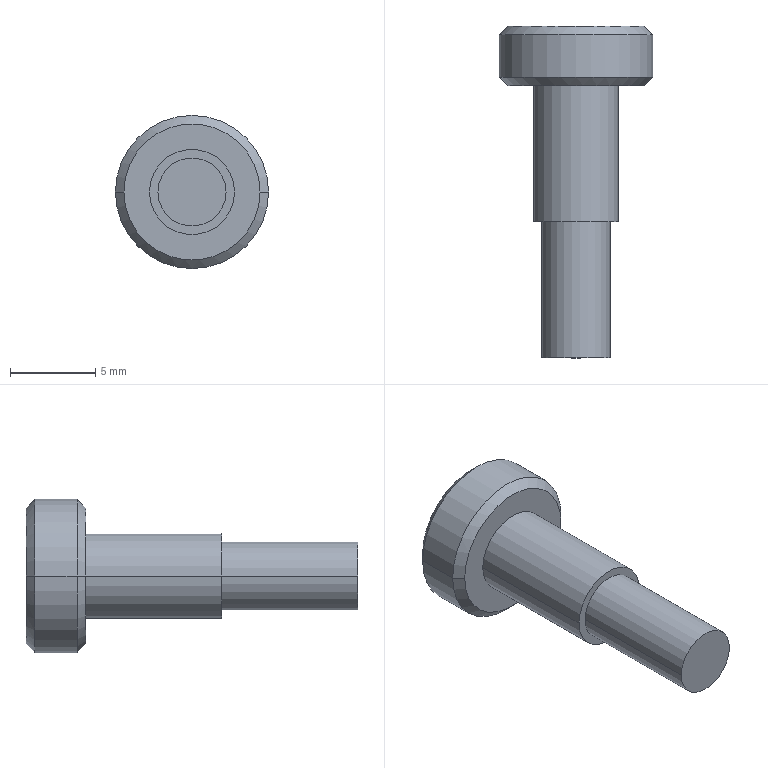Part | SolidWorks | features Attribute 3, Chamfer 1, ICE 1, Revolution 1 | 1 solid | 21 faces | box 9 x 19.5 x 9 mm | volume 457.876 mm3 | plane 11 | cylinder 6 | cone 4 | commonest cylinder face diameters 4 x2 5 x2 9 x2
STEP:
#1=CARTESIAN_POINT('',(-4.,19.5,0.));
#2=VERTEX_POINT('',#1);
#3=CARTESIAN_POINT('',(4.,19.5,0.));
#4=VERTEX_POINT('',#3);
#5=CARTESIAN_POINT('',(0.,19.5,0.));
#6=DIRECTION('',(0.,1.,0.));
#7=DIRECTION('',(1.,0.,0.));
#8=AXIS2_PLACEMENT_3D('',#5,#6,#7);
#9=CIRCLE('',#8,4.);
#10=EDGE_CURVE('',#2,#4,#9,.T.);
#11=ORIENTED_EDGE('',*,*,#10,.F.);
#12=CARTESIAN_POINT('',(-4.5,19.,0.));
#13=VERTEX_POINT('',#12);
#14=CARTESIAN_POINT('',(-4.5,19.,0.));
#15=DIRECTION('',(-0.7071,-0.7071,0.));
#16=VECTOR('',#15,1000.);
#17=LINE('',#14,#16);
#18=EDGE_CURVE('',#2,#13,#17,.T.);
#19=ORIENTED_EDGE('',*,*,#18,.T.);
#20=CARTESIAN_POINT('',(4.5,19.,0.));
#21=VERTEX_POINT('',#20);
#22=CARTESIAN_POINT('',(0.,19.,0.));
#23=DIRECTION('',(0.,-1.,0.));
#24=DIRECTION('',(1.,0.,0.));
#25=AXIS2_PLACEMENT_3D('',#22,#23,#24);
#26=CIRCLE('',#25,4.5);
#27=EDGE_CURVE('',#21,#13,#26,.T.);
#28=ORIENTED_EDGE('',*,*,#27,.F.);
#29=CARTESIAN_POINT('',(4.5,19.,0.));
#30=DIRECTION('',(0.7071,-0.7071,0.));
#31=VECTOR('',#30,1000.);
#32=LINE('',#29,#31);
#33=EDGE_CURVE('',#4,#21,#32,.T.);
#34=ORIENTED_EDGE('',*,*,#33,.F.);
#35=EDGE_LOOP('',(#11,#19,#28,#34));
#36=FACE_OUTER_BOUND('',#35,.T.);
#37=CARTESIAN_POINT('',(0.,19.,0.));
#38=DIRECTION('',(0.,-1.,0.));
#39=DIRECTION('',(1.,0.,0.));
#40=AXIS2_PLACEMENT_3D('',#37,#38,#39);
#41=CONICAL_SURFACE('',#40,4.5,0.7854);
#42=ADVANCED_FACE('',(#36),#41,.T.);
#43=CARTESIAN_POINT('',(4.,16.,0.));
#44=VERTEX_POINT('',#43);
#45=CARTESIAN_POINT('',(-4.,16.,0.));
#46=VERTEX_POINT('',#45);
#47=CARTESIAN_POINT('',(0.,16.,0.));
#48=DIRECTION('',(0.,-1.,0.));
#49=DIRECTION('',(-1.,0.,0.));
#50=AXIS2_PLACEMENT_3D('',#47,#48,#49);
#51=CIRCLE('',#50,4.);
#52=EDGE_CURVE('',#44,#46,#51,.T.);
#53=ORIENTED_EDGE('',*,*,#52,.F.);
#54=CARTESIAN_POINT('',(4.5,16.5,0.));
#55=VERTEX_POINT('',#54);
#56=CARTESIAN_POINT('',(4.,16.,0.));
#57=DIRECTION('',(0.7071,0.7071,0.));
#58=VECTOR('',#57,1000.);
#59=LINE('',#56,#58);
#60=EDGE_CURVE('',#44,#55,#59,.T.);
#61=ORIENTED_EDGE('',*,*,#60,.T.);
#62=CARTESIAN_POINT('',(-4.5,16.5,0.));
#63=VERTEX_POINT('',#62);
#64=CARTESIAN_POINT('',(0.,16.5,0.));
#65=DIRECTION('',(0.,1.,0.));
#66=DIRECTION('',(-1.,0.,0.));
#67=AXIS2_PLACEMENT_3D('',#64,#65,#66);
#68=CIRCLE('',#67,4.5);
#69=EDGE_CURVE('',#63,#55,#68,.T.);
#70=ORIENTED_EDGE('',*,*,#69,.F.);
#71=CARTESIAN_POINT('',(-4.,16.,0.));
#72=DIRECTION('',(-0.7071,0.7071,0.));
#73=VECTOR('',#72,1000.);
#74=LINE('',#71,#73);
#75=EDGE_CURVE('',#46,#63,#74,.T.);
#76=ORIENTED_EDGE('',*,*,#75,.F.);
#77=EDGE_LOOP('',(#53,#61,#70,#76));
#78=FACE_OUTER_BOUND('',#77,.T.);
#79=CARTESIAN_POINT('',(0.,16.,0.));
#80=DIRECTION('',(0.,1.,0.));
#81=DIRECTION('',(-1.,0.,0.));
#82=AXIS2_PLACEMENT_3D('',#79,#80,#81);
#83=CONICAL_SURFACE('',#82,4.,0.7854);
#84=ADVANCED_FACE('',(#78),#83,.T.);
#85=CARTESIAN_POINT('',(2.,8.,0.));
#86=VERTEX_POINT('',#85);
#87=CARTESIAN_POINT('',(-2.,8.,0.));
#88=VERTEX_POINT('',#87);
#89=CARTESIAN_POINT('',(0.,8.,0.));
#90=DIRECTION('',(0.,-1.,0.));
#91=DIRECTION('',(1.,0.,0.));
#92=AXIS2_PLACEMENT_3D('',#89,#90,#91);
#93=CIRCLE('',#92,2.);
#94=EDGE_CURVE('',#86,#88,#93,.T.);
#95=ORIENTED_EDGE('',*,*,#94,.T.);
#96=CARTESIAN_POINT('',(-2.,0.,0.));
#97=VERTEX_POINT('',#96);
#98=CARTESIAN_POINT('',(-2.,0.,0.));
#99=DIRECTION('',(0.,-1.,0.));
#100=VECTOR('',#99,1000.);
#101=LINE('',#98,#100);
#102=EDGE_CURVE('',#88,#97,#101,.T.);
#103=ORIENTED_EDGE('',*,*,#102,.T.);
#104=CARTESIAN_POINT('',(2.,0.,0.));
#105=VERTEX_POINT('',#104);
#106=CARTESIAN_POINT('',(0.,0.,0.));
#107=DIRECTION('',(0.,-1.,0.));
#108=DIRECTION('',(1.,0.,0.));
#109=AXIS2_PLACEMENT_3D('',#106,#107,#108);
#110=CIRCLE('',#109,2.);
#111=EDGE_CURVE('',#105,#97,#110,.T.);
#112=ORIENTED_EDGE('',*,*,#111,.F.);
#113=CARTESIAN_POINT('',(2.,0.,0.));
#114=DIRECTION('',(0.,-1.,0.));
#115=VECTOR('',#114,1000.);
#116=LINE('',#113,#115);
#117=EDGE_CURVE('',#86,#105,#116,.T.);
#118=ORIENTED_EDGE('',*,*,#117,.F.);
#119=EDGE_LOOP('',(#95,#103,#112,#118));
#120=FACE_OUTER_BOUND('',#119,.T.);
#121=CARTESIAN_POINT('',(0.,0.,0.));
#122=DIRECTION('',(0.,-1.,0.));
#123=DIRECTION('',(1.,0.,0.));
#124=AXIS2_PLACEMENT_3D('',#121,#122,#123);
#125=CYLINDRICAL_SURFACE('',#124,2.);
#126=ADVANCED_FACE('',(#120),#125,.T.);
#127=CARTESIAN_POINT('',(2.5,16.,0.));
#128=VERTEX_POINT('',#127);
#129=CARTESIAN_POINT('',(-2.5,16.,0.));
#130=VERTEX_POINT('',#129);
#131=CARTESIAN_POINT('',(0.,16.,0.));
#132=DIRECTION('',(0.,-1.,0.));
#133=DIRECTION('',(1.,0.,0.));
#134=AXIS2_PLACEMENT_3D('',#131,#132,#133);
#135=CIRCLE('',#134,2.5);
#136=EDGE_CURVE('',#128,#130,#135,.T.);
#137=ORIENTED_EDGE('',*,*,#136,.T.);
#138=CARTESIAN_POINT('',(-2.5,8.,0.));
#139=VERTEX_POINT('',#138);
#140=CARTESIAN_POINT('',(-2.5,0.,0.));
#141=DIRECTION('',(0.,-1.,0.));
#142=VECTOR('',#141,1000.);
#143=LINE('',#140,#142);
#144=EDGE_CURVE('',#130,#139,#143,.T.);
#145=ORIENTED_EDGE('',*,*,#144,.T.);
#146=CARTESIAN_POINT('',(2.5,8.,0.));
#147=VERTEX_POINT('',#146);
#148=CARTESIAN_POINT('',(0.,8.,0.));
#149=DIRECTION('',(0.,-1.,0.));
#150=DIRECTION('',(1.,0.,0.));
#151=AXIS2_PLACEMENT_3D('',#148,#149,#150);
#152=CIRCLE('',#151,2.5);
#153=EDGE_CURVE('',#147,#139,#152,.T.);
#154=ORIENTED_EDGE('',*,*,#153,.F.);
#155=CARTESIAN_POINT('',(2.5,0.,0.));
#156=DIRECTION('',(0.,-1.,0.));
#157=VECTOR('',#156,1000.);
#158=LINE('',#155,#157);
#159=EDGE_CURVE('',#128,#147,#158,.T.);
#160=ORIENTED_EDGE('',*,*,#159,.F.);
#161=EDGE_LOOP('',(#137,#145,#154,#160));
#162=FACE_OUTER_BOUND('',#161,.T.);
#163=CARTESIAN_POINT('',(0.,0.,0.));
#164=DIRECTION('',(0.,-1.,0.));
#165=DIRECTION('',(1.,0.,0.));
#166=AXIS2_PLACEMENT_3D('',#163,#164,#165);
#167=CYLINDRICAL_SURFACE('',#166,2.5);
#168=ADVANCED_FACE('',(#162),#167,.T.);
#169=ORIENTED_EDGE('',*,*,#27,.T.);
#170=CARTESIAN_POINT('',(-4.5,0.,0.));
#171=DIRECTION('',(0.,-1.,0.));
#172=VECTOR('',#171,1000.);
#173=LINE('',#170,#172);
#174=EDGE_CURVE('',#13,#63,#173,.T.);
#175=ORIENTED_EDGE('',*,*,#174,.T.);
#176=ORIENTED_EDGE('',*,*,#69,.T.);
#177=CARTESIAN_POINT('',(4.5,0.,0.));
#178=DIRECTION('',(0.,-1.,0.));
#179=VECTOR('',#178,1000.);
#180=LINE('',#177,#179);
#181=EDGE_CURVE('',#21,#55,#180,.T.);
#182=ORIENTED_EDGE('',*,*,#181,.F.);
#183=EDGE_LOOP('',(#169,#175,#176,#182));
#184=FACE_OUTER_BOUND('',#183,.T.);
#185=CARTESIAN_POINT('',(0.,0.,0.));
#186=DIRECTION('',(0.,-1.,0.));
#187=DIRECTION('',(1.,0.,0.));
#188=AXIS2_PLACEMENT_3D('',#185,#186,#187);
#189=CYLINDRICAL_SURFACE('',#188,4.5);
#190=ADVANCED_FACE('',(#184),#189,.T.);
#191=ORIENTED_EDGE('',*,*,#111,.T.);
#192=CARTESIAN_POINT('',(0.,0.,0.));
#193=DIRECTION('',(0.,-1.,0.));
#194=DIRECTION('',(1.,0.,0.));
#195=AXIS2_PLACEMENT_3D('',#192,#193,#194);
#196=CIRCLE('',#195,2.);
#197=EDGE_CURVE('',#97,#105,#196,.T.);
#198=ORIENTED_EDGE('',*,*,#197,.T.);
#199=EDGE_LOOP('',(#191,#198));
#200=FACE_OUTER_BOUND('',#199,.T.);
#201=CARTESIAN_POINT('',(-2.,0.,0.));
#202=DIRECTION('',(0.,1.,0.));
#203=DIRECTION('',(-1.,0.,0.));
#204=AXIS2_PLACEMENT_3D('',#201,#202,#203);
#205=PLANE('',#204);
#206=ADVANCED_FACE('',(#200),#205,.F.);
#207=CARTESIAN_POINT('',(0.,19.5,0.));
#208=DIRECTION('',(0.,1.,0.));
#209=DIRECTION('',(1.,0.,0.));
#210=AXIS2_PLACEMENT_3D('',#207,#208,#209);
#211=CIRCLE('',#210,4.);
#212=EDGE_CURVE('',#4,#2,#211,.T.);
#213=ORIENTED_EDGE('',*,*,#212,.T.);
#214=ORIENTED_EDGE('',*,*,#10,.T.);
#215=EDGE_LOOP('',(#213,#214));
#216=FACE_OUTER_BOUND('',#215,.T.);
#217=CARTESIAN_POINT('',(1.51,19.5,-0.8492));
#218=VERTEX_POINT('',#217);
#219=CARTESIAN_POINT('',(0.01932,19.5,-1.732));
#220=VERTEX_POINT('',#219);
#221=CARTESIAN_POINT('',(1.51,19.5,-0.8492));
#222=DIRECTION('',(-0.8604,0.,-0.5096));
#223=VECTOR('',#222,1000.);
#224=LINE('',#221,#223);
#225=EDGE_CURVE('',#218,#220,#224,.T.);
#226=ORIENTED_EDGE('',*,*,#225,.F.);
#227=CARTESIAN_POINT('',(1.49,19.5,0.8827));
#228=VERTEX_POINT('',#227);
#229=CARTESIAN_POINT('',(1.49,19.5,0.8827));
#230=DIRECTION('',(0.01115,0.,-0.9999));
#231=VECTOR('',#230,1000.);
#232=LINE('',#229,#231);
#233=EDGE_CURVE('',#228,#218,#232,.T.);
#234=ORIENTED_EDGE('',*,*,#233,.F.);
#235=CARTESIAN_POINT('',(-0.01932,19.5,1.732));
#236=VERTEX_POINT('',#235);
#237=CARTESIAN_POINT('',(-0.01932,19.5,1.732));
#238=DIRECTION('',(0.8715,0.,-0.4903));
#239=VECTOR('',#238,1000.);
#240=LINE('',#237,#239);
#241=EDGE_CURVE('',#236,#228,#240,.T.);
#242=ORIENTED_EDGE('',*,*,#241,.F.);
#243=CARTESIAN_POINT('',(-1.51,19.5,0.8492));
#244=VERTEX_POINT('',#243);
#245=CARTESIAN_POINT('',(-1.51,19.5,0.8492));
#246=DIRECTION('',(0.8604,0.,0.5096));
#247=VECTOR('',#246,1000.);
#248=LINE('',#245,#247);
#249=EDGE_CURVE('',#244,#236,#248,.T.);
#250=ORIENTED_EDGE('',*,*,#249,.F.);
#251=CARTESIAN_POINT('',(-1.49,19.5,-0.8827));
#252=VERTEX_POINT('',#251);
#253=CARTESIAN_POINT('',(-1.49,19.5,-0.8827));
#254=DIRECTION('',(-0.01115,0.,0.9999));
#255=VECTOR('',#254,1000.);
#256=LINE('',#253,#255);
#257=EDGE_CURVE('',#252,#244,#256,.T.);
#258=ORIENTED_EDGE('',*,*,#257,.F.);
#259=CARTESIAN_POINT('',(0.01932,19.5,-1.732));
#260=DIRECTION('',(-0.8715,0.,0.4903));
#261=VECTOR('',#260,1000.);
#262=LINE('',#259,#261);
#263=EDGE_CURVE('',#220,#252,#262,.T.);
#264=ORIENTED_EDGE('',*,*,#263,.F.);
#265=EDGE_LOOP('',(#226,#234,#242,#250,#258,#264));
#266=FACE_BOUND('',#265,.T.);
#267=CARTESIAN_POINT('',(0.,19.5,0.));
#268=DIRECTION('',(0.,-1.,0.));
#269=DIRECTION('',(1.,0.,0.));
#270=AXIS2_PLACEMENT_3D('',#267,#268,#269);
#271=PLANE('',#270);
#272=ADVANCED_FACE('',(#216,#266),#271,.F.);
#273=ORIENTED_EDGE('',*,*,#174,.F.);
#274=CARTESIAN_POINT('',(0.,19.,0.));
#275=DIRECTION('',(0.,-1.,0.));
#276=DIRECTION('',(1.,0.,0.));
#277=AXIS2_PLACEMENT_3D('',#274,#275,#276);
#278=CIRCLE('',#277,4.5);
#279=EDGE_CURVE('',#13,#21,#278,.T.);
#280=ORIENTED_EDGE('',*,*,#279,.T.);
#281=ORIENTED_EDGE('',*,*,#181,.T.);
#282=CARTESIAN_POINT('',(0.,16.5,0.));
#283=DIRECTION('',(0.,1.,0.));
#284=DIRECTION('',(-1.,0.,0.));
#285=AXIS2_PLACEMENT_3D('',#282,#283,#284);
#286=CIRCLE('',#285,4.5);
#287=EDGE_CURVE('',#55,#63,#286,.T.);
#288=ORIENTED_EDGE('',*,*,#287,.T.);
#289=EDGE_LOOP('',(#273,#280,#281,#288));
#290=FACE_OUTER_BOUND('',#289,.T.);
#291=CARTESIAN_POINT('',(0.,0.,0.));
#292=DIRECTION('',(0.,-1.,0.));
#293=DIRECTION('',(1.,0.,0.));
#294=AXIS2_PLACEMENT_3D('',#291,#292,#293);
#295=CYLINDRICAL_SURFACE('',#294,4.5);
#296=ADVANCED_FACE('',(#290),#295,.T.);
#297=CARTESIAN_POINT('',(0.,16.,0.));
#298=DIRECTION('',(0.,-1.,0.));
#299=DIRECTION('',(-1.,0.,0.));
#300=AXIS2_PLACEMENT_3D('',#297,#298,#299);
#301=CIRCLE('',#300,4.);
#302=EDGE_CURVE('',#46,#44,#301,.T.);
#303=ORIENTED_EDGE('',*,*,#302,.T.);
#304=ORIENTED_EDGE('',*,*,#52,.T.);
#305=EDGE_LOOP('',(#303,#304));
#306=FACE_OUTER_BOUND('',#305,.T.);
#307=ORIENTED_EDGE('',*,*,#136,.F.);
#308=CARTESIAN_POINT('',(0.,16.,0.));
#309=DIRECTION('',(0.,-1.,0.));
#310=DIRECTION('',(1.,0.,0.));
#311=AXIS2_PLACEMENT_3D('',#308,#309,#310);
#312=CIRCLE('',#311,2.5);
#313=EDGE_CURVE('',#130,#128,#312,.T.);
#314=ORIENTED_EDGE('',*,*,#313,.F.);
#315=EDGE_LOOP('',(#307,#314));
#316=FACE_BOUND('',#315,.T.);
#317=CARTESIAN_POINT('',(-4.5,16.,0.));
#318=DIRECTION('',(0.,1.,0.));
#319=DIRECTION('',(-1.,0.,0.));
#320=AXIS2_PLACEMENT_3D('',#317,#318,#319);
#321=PLANE('',#320);
#322=ADVANCED_FACE('',(#306,#316),#321,.F.);
#323=ORIENTED_EDGE('',*,*,#144,.F.);
#324=ORIENTED_EDGE('',*,*,#313,.T.);
#325=ORIENTED_EDGE('',*,*,#159,.T.);
#326=CARTESIAN_POINT('',(0.,8.,0.));
#327=DIRECTION('',(0.,-1.,0.));
#328=DIRECTION('',(1.,0.,0.));
#329=AXIS2_PLACEMENT_3D('',#326,#327,#328);
#330=CIRCLE('',#329,2.5);
#331=EDGE_CURVE('',#139,#147,#330,.T.);
#332=ORIENTED_EDGE('',*,*,#331,.F.);
#333=EDGE_LOOP('',(#323,#324,#325,#332));
#334=FACE_OUTER_BOUND('',#333,.T.);
#335=CARTESIAN_POINT('',(0.,0.,0.));
#336=DIRECTION('',(0.,-1.,0.));
#337=DIRECTION('',(1.,0.,0.));
#338=AXIS2_PLACEMENT_3D('',#335,#336,#337);
#339=CYLINDRICAL_SURFACE('',#338,2.5);
#340=ADVANCED_FACE('',(#334),#339,.T.);
#341=ORIENTED_EDGE('',*,*,#94,.F.);
#342=CARTESIAN_POINT('',(0.,8.,0.));
#343=DIRECTION('',(0.,-1.,0.));
#344=DIRECTION('',(1.,0.,0.));
#345=AXIS2_PLACEMENT_3D('',#342,#343,#344);
#346=CIRCLE('',#345,2.);
#347=EDGE_CURVE('',#88,#86,#346,.T.);
#348=ORIENTED_EDGE('',*,*,#347,.F.);
#349=EDGE_LOOP('',(#341,#348));
#350=FACE_BOUND('',#349,.T.);
#351=ORIENTED_EDGE('',*,*,#153,.T.);
#352=ORIENTED_EDGE('',*,*,#331,.T.);
#353=EDGE_LOOP('',(#351,#352));
#354=FACE_OUTER_BOUND('',#353,.T.);
#355=CARTESIAN_POINT('',(-2.5,8.,0.));
#356=DIRECTION('',(0.,1.,0.));
#357=DIRECTION('',(-1.,0.,0.));
#358=AXIS2_PLACEMENT_3D('',#355,#356,#357);
#359=PLANE('',#358);
#360=ADVANCED_FACE('',(#350,#354),#359,.F.);
#361=ORIENTED_EDGE('',*,*,#102,.F.);
#362=ORIENTED_EDGE('',*,*,#347,.T.);
#363=ORIENTED_EDGE('',*,*,#117,.T.);
#364=ORIENTED_EDGE('',*,*,#197,.F.);
#365=EDGE_LOOP('',(#361,#362,#363,#364));
#366=FACE_OUTER_BOUND('',#365,.T.);
#367=CARTESIAN_POINT('',(0.,0.,0.));
#368=DIRECTION('',(0.,-1.,0.));
#369=DIRECTION('',(1.,0.,0.));
#370=AXIS2_PLACEMENT_3D('',#367,#368,#369);
#371=CYLINDRICAL_SURFACE('',#370,2.);
#372=ADVANCED_FACE('',(#366),#371,.T.);
#373=ORIENTED_EDGE('',*,*,#233,.T.);
#374=CARTESIAN_POINT('',(1.51,17.5,-0.8492));
#375=VERTEX_POINT('',#374);
#376=CARTESIAN_POINT('',(1.51,17.5,-0.8492));
#377=DIRECTION('',(0.,1.,0.));
#378=VECTOR('',#377,1000.);
#379=LINE('',#376,#378);
#380=EDGE_CURVE('',#375,#218,#379,.T.);
#381=ORIENTED_EDGE('',*,*,#380,.F.);
#382=CARTESIAN_POINT('',(1.49,17.5,0.8827));
#383=VERTEX_POINT('',#382);
#384=CARTESIAN_POINT('',(1.49,17.5,0.8827));
#385=DIRECTION('',(0.01115,0.,-0.9999));
#386=VECTOR('',#385,1000.);
#387=LINE('',#384,#386);
#388=EDGE_CURVE('',#383,#375,#387,.T.);
#389=ORIENTED_EDGE('',*,*,#388,.F.);
#390=CARTESIAN_POINT('',(1.49,17.5,0.8827));
#391=DIRECTION('',(0.,1.,0.));
#392=VECTOR('',#391,1000.);
#393=LINE('',#390,#392);
#394=EDGE_CURVE('',#383,#228,#393,.T.);
#395=ORIENTED_EDGE('',*,*,#394,.T.);
#396=EDGE_LOOP('',(#373,#381,#389,#395));
#397=FACE_OUTER_BOUND('',#396,.T.);
#398=CARTESIAN_POINT('',(1.49,17.5,0.8827));
#399=DIRECTION('',(0.9999,0.,0.01115));
#400=DIRECTION('',(0.01115,0.,-0.9999));
#401=AXIS2_PLACEMENT_3D('',#398,#399,#400);
#402=PLANE('',#401);
#403=ADVANCED_FACE('',(#397),#402,.F.);
#404=ORIENTED_EDGE('',*,*,#241,.T.);
#405=ORIENTED_EDGE('',*,*,#394,.F.);
#406=CARTESIAN_POINT('',(-0.01932,17.5,1.732));
#407=VERTEX_POINT('',#406);
#408=CARTESIAN_POINT('',(-0.01932,17.5,1.732));
#409=DIRECTION('',(0.8715,0.,-0.4903));
#410=VECTOR('',#409,1000.);
#411=LINE('',#408,#410);
#412=EDGE_CURVE('',#407,#383,#411,.T.);
#413=ORIENTED_EDGE('',*,*,#412,.F.);
#414=CARTESIAN_POINT('',(-0.01932,17.5,1.732));
#415=DIRECTION('',(0.,1.,0.));
#416=VECTOR('',#415,1000.);
#417=LINE('',#414,#416);
#418=EDGE_CURVE('',#407,#236,#417,.T.);
#419=ORIENTED_EDGE('',*,*,#418,.T.);
#420=EDGE_LOOP('',(#404,#405,#413,#419));
#421=FACE_OUTER_BOUND('',#420,.T.);
#422=CARTESIAN_POINT('',(-0.01932,17.5,1.732));
#423=DIRECTION('',(0.4903,0.,0.8715));
#424=DIRECTION('',(0.8715,0.,-0.4903));
#425=AXIS2_PLACEMENT_3D('',#422,#423,#424);
#426=PLANE('',#425);
#427=ADVANCED_FACE('',(#421),#426,.F.);
#428=ORIENTED_EDGE('',*,*,#249,.T.);
#429=ORIENTED_EDGE('',*,*,#418,.F.);
#430=CARTESIAN_POINT('',(-1.51,17.5,0.8492));
#431=VERTEX_POINT('',#430);
#432=CARTESIAN_POINT('',(-1.51,17.5,0.8492));
#433=DIRECTION('',(0.8604,0.,0.5096));
#434=VECTOR('',#433,1000.);
#435=LINE('',#432,#434);
#436=EDGE_CURVE('',#431,#407,#435,.T.);
#437=ORIENTED_EDGE('',*,*,#436,.F.);
#438=CARTESIAN_POINT('',(-1.51,17.5,0.8492));
#439=DIRECTION('',(0.,1.,0.));
#440=VECTOR('',#439,1000.);
#441=LINE('',#438,#440);
#442=EDGE_CURVE('',#431,#244,#441,.T.);
#443=ORIENTED_EDGE('',*,*,#442,.T.);
#444=EDGE_LOOP('',(#428,#429,#437,#443));
#445=FACE_OUTER_BOUND('',#444,.T.);
#446=CARTESIAN_POINT('',(-1.51,17.5,0.8492));
#447=DIRECTION('',(-0.5096,0.,0.8604));
#448=DIRECTION('',(0.8604,0.,0.5096));
#449=AXIS2_PLACEMENT_3D('',#446,#447,#448);
#450=PLANE('',#449);
#451=ADVANCED_FACE('',(#445),#450,.F.);
#452=ORIENTED_EDGE('',*,*,#257,.T.);
#453=ORIENTED_EDGE('',*,*,#442,.F.);
#454=CARTESIAN_POINT('',(-1.49,17.5,-0.8827));
#455=VERTEX_POINT('',#454);
#456=CARTESIAN_POINT('',(-1.49,17.5,-0.8827));
#457=DIRECTION('',(-0.01115,0.,0.9999));
#458=VECTOR('',#457,1000.);
#459=LINE('',#456,#458);
#460=EDGE_CURVE('',#455,#431,#459,.T.);
#461=ORIENTED_EDGE('',*,*,#460,.F.);
#462=CARTESIAN_POINT('',(-1.49,17.5,-0.8827));
#463=DIRECTION('',(0.,1.,0.));
#464=VECTOR('',#463,1000.);
#465=LINE('',#462,#464);
#466=EDGE_CURVE('',#455,#252,#465,.T.);
#467=ORIENTED_EDGE('',*,*,#466,.T.);
#468=EDGE_LOOP('',(#452,#453,#461,#467));
#469=FACE_OUTER_BOUND('',#468,.T.);
#470=CARTESIAN_POINT('',(-1.49,17.5,-0.8827));
#471=DIRECTION('',(-0.9999,0.,-0.01115));
#472=DIRECTION('',(-0.01115,0.,0.9999));
#473=AXIS2_PLACEMENT_3D('',#470,#471,#472);
#474=PLANE('',#473);
#475=ADVANCED_FACE('',(#469),#474,.F.);
#476=ORIENTED_EDGE('',*,*,#263,.T.);
#477=ORIENTED_EDGE('',*,*,#466,.F.);
#478=CARTESIAN_POINT('',(0.01932,17.5,-1.732));
#479=VERTEX_POINT('',#478);
#480=CARTESIAN_POINT('',(0.01932,17.5,-1.732));
#481=DIRECTION('',(-0.8715,0.,0.4903));
#482=VECTOR('',#481,1000.);
#483=LINE('',#480,#482);
#484=EDGE_CURVE('',#479,#455,#483,.T.);
#485=ORIENTED_EDGE('',*,*,#484,.F.);
#486=CARTESIAN_POINT('',(0.01932,17.5,-1.732));
#487=DIRECTION('',(0.,1.,0.));
#488=VECTOR('',#487,1000.);
#489=LINE('',#486,#488);
#490=EDGE_CURVE('',#479,#220,#489,.T.);
#491=ORIENTED_EDGE('',*,*,#490,.T.);
#492=EDGE_LOOP('',(#476,#477,#485,#491));
#493=FACE_OUTER_BOUND('',#492,.T.);
#494=CARTESIAN_POINT('',(0.01932,17.5,-1.732));
#495=DIRECTION('',(-0.4903,0.,-0.8715));
#496=DIRECTION('',(-0.8715,0.,0.4903));
#497=AXIS2_PLACEMENT_3D('',#494,#495,#496);
#498=PLANE('',#497);
#499=ADVANCED_FACE('',(#493),#498,.F.);
#500=ORIENTED_EDGE('',*,*,#225,.T.);
#501=ORIENTED_EDGE('',*,*,#490,.F.);
#502=CARTESIAN_POINT('',(1.51,17.5,-0.8492));
#503=DIRECTION('',(-0.8604,0.,-0.5096));
#504=VECTOR('',#503,1000.);
#505=LINE('',#502,#504);
#506=EDGE_CURVE('',#375,#479,#505,.T.);
#507=ORIENTED_EDGE('',*,*,#506,.F.);
#508=ORIENTED_EDGE('',*,*,#380,.T.);
#509=EDGE_LOOP('',(#500,#501,#507,#508));
#510=FACE_OUTER_BOUND('',#509,.T.);
#511=CARTESIAN_POINT('',(1.51,17.5,-0.8492));
#512=DIRECTION('',(0.5096,0.,-0.8604));
#513=DIRECTION('',(-0.8604,0.,-0.5096));
#514=AXIS2_PLACEMENT_3D('',#511,#512,#513);
#515=PLANE('',#514);
#516=ADVANCED_FACE('',(#510),#515,.F.);
#517=ORIENTED_EDGE('',*,*,#388,.T.);
#518=ORIENTED_EDGE('',*,*,#506,.T.);
#519=ORIENTED_EDGE('',*,*,#484,.T.);
#520=ORIENTED_EDGE('',*,*,#460,.T.);
#521=ORIENTED_EDGE('',*,*,#436,.T.);
#522=ORIENTED_EDGE('',*,*,#412,.T.);
#523=EDGE_LOOP('',(#517,#518,#519,#520,#521,#522));
#524=FACE_OUTER_BOUND('',#523,.T.);
#525=CARTESIAN_POINT('',(0.,17.5,0.));
#526=DIRECTION('',(0.,1.,0.));
#527=DIRECTION('',(0.,0.,1.));
#528=AXIS2_PLACEMENT_3D('',#525,#526,#527);
#529=PLANE('',#528);
#530=ADVANCED_FACE('',(#524),#529,.T.);
#531=ORIENTED_EDGE('',*,*,#60,.F.);
#532=ORIENTED_EDGE('',*,*,#302,.F.);
#533=ORIENTED_EDGE('',*,*,#75,.T.);
#534=ORIENTED_EDGE('',*,*,#287,.F.);
#535=EDGE_LOOP('',(#531,#532,#533,#534));
#536=FACE_OUTER_BOUND('',#535,.T.);
#537=CARTESIAN_POINT('',(0.,16.,0.));
#538=DIRECTION('',(0.,1.,0.));
#539=DIRECTION('',(-1.,0.,0.));
#540=AXIS2_PLACEMENT_3D('',#537,#538,#539);
#541=CONICAL_SURFACE('',#540,4.,0.7854);
#542=ADVANCED_FACE('',(#536),#541,.T.);
#543=ORIENTED_EDGE('',*,*,#18,.F.);
#544=ORIENTED_EDGE('',*,*,#212,.F.);
#545=ORIENTED_EDGE('',*,*,#33,.T.);
#546=ORIENTED_EDGE('',*,*,#279,.F.);
#547=EDGE_LOOP('',(#543,#544,#545,#546));
#548=FACE_OUTER_BOUND('',#547,.T.);
#549=CARTESIAN_POINT('',(0.,19.,0.));
#550=DIRECTION('',(0.,-1.,0.));
#551=DIRECTION('',(1.,0.,0.));
#552=AXIS2_PLACEMENT_3D('',#549,#550,#551);
#553=CONICAL_SURFACE('',#552,4.5,0.7854);
#554=ADVANCED_FACE('',(#548),#553,.T.);
#555=CLOSED_SHELL('',(#42,#84,#126,#168,#190,#206,#272,#296,#322,#340,#360,#372,#403,#427,#451,#475,#499,#516,#530,#542,#554));
#556=MANIFOLD_SOLID_BREP('',#555);
#557=CARTESIAN_POINT('',(0.,0.,0.));
#558=DIRECTION('',(0.,0.,1.));
#559=DIRECTION('',(1.,0.,0.));
#560=AXIS2_PLACEMENT_3D('',#557,#558,#559);
#561=(LENGTH_UNIT()NAMED_UNIT(*)SI_UNIT(.MILLI.,.METRE.));
#562=UNCERTAINTY_MEASURE_WITH_UNIT(LENGTH_MEASURE(0.00001),#561,'','');
#563=(NAMED_UNIT(*)PLANE_ANGLE_UNIT()SI_UNIT($,.RADIAN.));
#564=(NAMED_UNIT(*)SI_UNIT($,.STERADIAN.)SOLID_ANGLE_UNIT());
#565=(GEOMETRIC_REPRESENTATION_CONTEXT(3)GLOBAL_UNCERTAINTY_ASSIGNED_CONTEXT((#562))GLOBAL_UNIT_ASSIGNED_CONTEXT((#561,#563,#564))REPRESENTATION_CONTEXT('',''));
#566=ADVANCED_BREP_SHAPE_REPRESENTATION('',(#556,#560),#565);